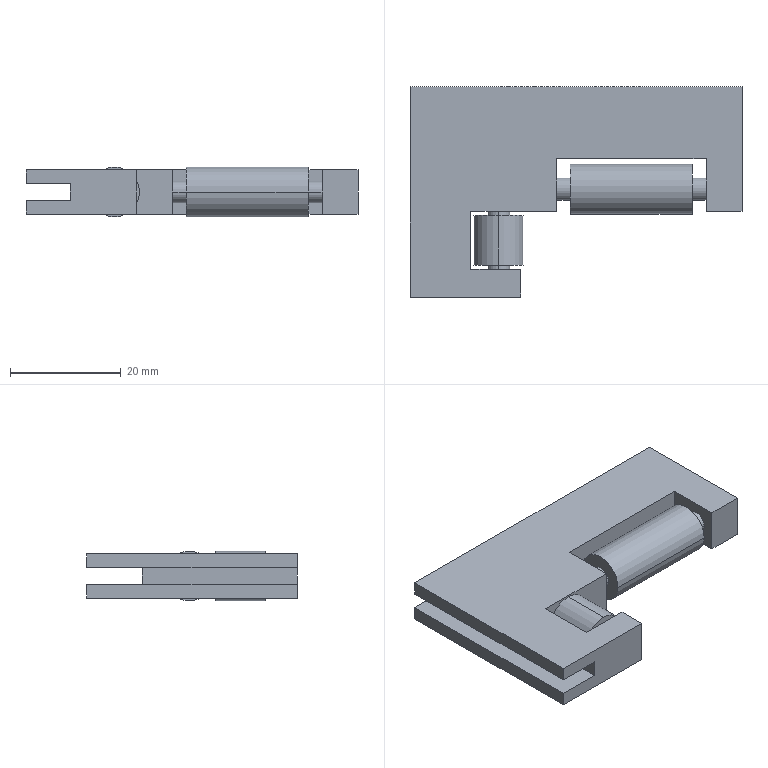Part | STEP file | T Slider Block | 3 solids | 40 faces | box 60 x 38 x 9 mm | volume 10054 mm3 | plane 28 | cylinder 12 | commonest cylinder face diameters 4 x8 9 x4
STEP:
#1=CARTESIAN_POINT('',(-41.818,-4.436,-4.5));
#2=VERTEX_POINT('',#1);
#3=CARTESIAN_POINT('',(-41.818,-4.436,4.5));
#4=VERTEX_POINT('',#3);
#5=CARTESIAN_POINT('',(-41.818,-4.436,0.));
#6=DIRECTION('',(0.,-1.,0.));
#7=DIRECTION('',(0.,0.,-1.));
#8=AXIS2_PLACEMENT_3D('',#5,#6,#7);
#9=CIRCLE('',#8,4.5);
#10=EDGE_CURVE('',#2,#4,#9,.T.);
#11=ORIENTED_EDGE('',*,*,#10,.T.);
#12=CARTESIAN_POINT('',(-41.818,-13.436,4.5));
#13=VERTEX_POINT('',#12);
#14=CARTESIAN_POINT('',(-41.818,-14.186,4.5));
#15=DIRECTION('',(0.,-1.,0.));
#16=VECTOR('',#15,1000.);
#17=LINE('',#14,#16);
#18=EDGE_CURVE('',#4,#13,#17,.T.);
#19=ORIENTED_EDGE('',*,*,#18,.T.);
#20=CARTESIAN_POINT('',(-41.818,-13.436,-4.5));
#21=VERTEX_POINT('',#20);
#22=CARTESIAN_POINT('',(-41.818,-13.436,0.));
#23=DIRECTION('',(0.,1.,0.));
#24=DIRECTION('',(0.,0.,-1.));
#25=AXIS2_PLACEMENT_3D('',#22,#23,#24);
#26=CIRCLE('',#25,4.5);
#27=EDGE_CURVE('',#13,#21,#26,.T.);
#28=ORIENTED_EDGE('',*,*,#27,.T.);
#29=CARTESIAN_POINT('',(-41.818,-14.186,-4.5));
#30=DIRECTION('',(0.,-1.,0.));
#31=VECTOR('',#30,1000.);
#32=LINE('',#29,#31);
#33=EDGE_CURVE('',#2,#21,#32,.T.);
#34=ORIENTED_EDGE('',*,*,#33,.F.);
#35=EDGE_LOOP('',(#11,#19,#28,#34));
#36=FACE_OUTER_BOUND('',#35,.T.);
#37=CARTESIAN_POINT('',(-41.818,-14.186,0.));
#38=DIRECTION('',(0.,-1.,0.));
#39=DIRECTION('',(0.,0.,-1.));
#40=AXIS2_PLACEMENT_3D('',#37,#38,#39);
#41=CYLINDRICAL_SURFACE('',#40,4.5);
#42=ADVANCED_FACE('',(#36),#41,.T.);
#43=CARTESIAN_POINT('',(-41.818,-13.436,-2.));
#44=VERTEX_POINT('',#43);
#45=CARTESIAN_POINT('',(-41.818,-13.436,2.));
#46=VERTEX_POINT('',#45);
#47=CARTESIAN_POINT('',(-41.818,-13.436,0.));
#48=DIRECTION('',(0.,-1.,0.));
#49=DIRECTION('',(0.,0.,-1.));
#50=AXIS2_PLACEMENT_3D('',#47,#48,#49);
#51=CIRCLE('',#50,2.);
#52=EDGE_CURVE('',#44,#46,#51,.T.);
#53=ORIENTED_EDGE('',*,*,#52,.T.);
#54=CARTESIAN_POINT('',(-41.818,-14.186,2.));
#55=VERTEX_POINT('',#54);
#56=CARTESIAN_POINT('',(-41.818,-14.186,2.));
#57=DIRECTION('',(0.,-1.,0.));
#58=VECTOR('',#57,1000.);
#59=LINE('',#56,#58);
#60=EDGE_CURVE('',#46,#55,#59,.T.);
#61=ORIENTED_EDGE('',*,*,#60,.T.);
#62=CARTESIAN_POINT('',(-41.818,-14.186,-2.));
#63=VERTEX_POINT('',#62);
#64=CARTESIAN_POINT('',(-41.818,-14.186,0.));
#65=DIRECTION('',(0.,1.,0.));
#66=DIRECTION('',(0.,0.,-1.));
#67=AXIS2_PLACEMENT_3D('',#64,#65,#66);
#68=CIRCLE('',#67,2.);
#69=EDGE_CURVE('',#55,#63,#68,.T.);
#70=ORIENTED_EDGE('',*,*,#69,.T.);
#71=CARTESIAN_POINT('',(-41.818,-14.186,-2.));
#72=DIRECTION('',(0.,-1.,0.));
#73=VECTOR('',#72,1000.);
#74=LINE('',#71,#73);
#75=EDGE_CURVE('',#44,#63,#74,.T.);
#76=ORIENTED_EDGE('',*,*,#75,.F.);
#77=EDGE_LOOP('',(#53,#61,#70,#76));
#78=FACE_OUTER_BOUND('',#77,.T.);
#79=CARTESIAN_POINT('',(-41.818,-14.186,0.));
#80=DIRECTION('',(0.,-1.,0.));
#81=DIRECTION('',(0.,0.,-1.));
#82=AXIS2_PLACEMENT_3D('',#79,#80,#81);
#83=CYLINDRICAL_SURFACE('',#82,2.);
#84=ADVANCED_FACE('',(#78),#83,.T.);
#85=CARTESIAN_POINT('',(-41.818,-3.686,-2.));
#86=VERTEX_POINT('',#85);
#87=CARTESIAN_POINT('',(-41.818,-3.686,2.));
#88=VERTEX_POINT('',#87);
#89=CARTESIAN_POINT('',(-41.818,-3.686,0.));
#90=DIRECTION('',(0.,-1.,0.));
#91=DIRECTION('',(0.,0.,-1.));
#92=AXIS2_PLACEMENT_3D('',#89,#90,#91);
#93=CIRCLE('',#92,2.);
#94=EDGE_CURVE('',#86,#88,#93,.T.);
#95=ORIENTED_EDGE('',*,*,#94,.T.);
#96=CARTESIAN_POINT('',(-41.818,-4.436,2.));
#97=VERTEX_POINT('',#96);
#98=CARTESIAN_POINT('',(-41.818,-14.186,2.));
#99=DIRECTION('',(0.,-1.,0.));
#100=VECTOR('',#99,1000.);
#101=LINE('',#98,#100);
#102=EDGE_CURVE('',#88,#97,#101,.T.);
#103=ORIENTED_EDGE('',*,*,#102,.T.);
#104=CARTESIAN_POINT('',(-41.818,-4.436,-2.));
#105=VERTEX_POINT('',#104);
#106=CARTESIAN_POINT('',(-41.818,-4.436,0.));
#107=DIRECTION('',(0.,1.,0.));
#108=DIRECTION('',(0.,0.,-1.));
#109=AXIS2_PLACEMENT_3D('',#106,#107,#108);
#110=CIRCLE('',#109,2.);
#111=EDGE_CURVE('',#97,#105,#110,.T.);
#112=ORIENTED_EDGE('',*,*,#111,.T.);
#113=CARTESIAN_POINT('',(-41.818,-14.186,-2.));
#114=DIRECTION('',(0.,-1.,0.));
#115=VECTOR('',#114,1000.);
#116=LINE('',#113,#115);
#117=EDGE_CURVE('',#86,#105,#116,.T.);
#118=ORIENTED_EDGE('',*,*,#117,.F.);
#119=EDGE_LOOP('',(#95,#103,#112,#118));
#120=FACE_OUTER_BOUND('',#119,.T.);
#121=CARTESIAN_POINT('',(-41.818,-14.186,0.));
#122=DIRECTION('',(0.,-1.,0.));
#123=DIRECTION('',(0.,0.,-1.));
#124=AXIS2_PLACEMENT_3D('',#121,#122,#123);
#125=CYLINDRICAL_SURFACE('',#124,2.);
#126=ADVANCED_FACE('',(#120),#125,.T.);
#127=ORIENTED_EDGE('',*,*,#18,.F.);
#128=CARTESIAN_POINT('',(-41.818,-4.436,0.));
#129=DIRECTION('',(0.,-1.,0.));
#130=DIRECTION('',(0.,0.,-1.));
#131=AXIS2_PLACEMENT_3D('',#128,#129,#130);
#132=CIRCLE('',#131,4.5);
#133=EDGE_CURVE('',#4,#2,#132,.T.);
#134=ORIENTED_EDGE('',*,*,#133,.T.);
#135=ORIENTED_EDGE('',*,*,#33,.T.);
#136=CARTESIAN_POINT('',(-41.818,-13.436,0.));
#137=DIRECTION('',(0.,1.,0.));
#138=DIRECTION('',(0.,0.,-1.));
#139=AXIS2_PLACEMENT_3D('',#136,#137,#138);
#140=CIRCLE('',#139,4.5);
#141=EDGE_CURVE('',#21,#13,#140,.T.);
#142=ORIENTED_EDGE('',*,*,#141,.T.);
#143=EDGE_LOOP('',(#127,#134,#135,#142));
#144=FACE_OUTER_BOUND('',#143,.T.);
#145=CARTESIAN_POINT('',(-41.818,-14.186,0.));
#146=DIRECTION('',(0.,-1.,0.));
#147=DIRECTION('',(0.,0.,-1.));
#148=AXIS2_PLACEMENT_3D('',#145,#146,#147);
#149=CYLINDRICAL_SURFACE('',#148,4.5);
#150=ADVANCED_FACE('',(#144),#149,.T.);
#151=ORIENTED_EDGE('',*,*,#141,.F.);
#152=ORIENTED_EDGE('',*,*,#27,.F.);
#153=EDGE_LOOP('',(#151,#152));
#154=FACE_OUTER_BOUND('',#153,.T.);
#155=ORIENTED_EDGE('',*,*,#52,.F.);
#156=CARTESIAN_POINT('',(-41.818,-13.436,0.));
#157=DIRECTION('',(0.,-1.,0.));
#158=DIRECTION('',(0.,0.,-1.));
#159=AXIS2_PLACEMENT_3D('',#156,#157,#158);
#160=CIRCLE('',#159,2.);
#161=EDGE_CURVE('',#46,#44,#160,.T.);
#162=ORIENTED_EDGE('',*,*,#161,.F.);
#163=EDGE_LOOP('',(#155,#162));
#164=FACE_BOUND('',#163,.T.);
#165=CARTESIAN_POINT('',(-46.318,-13.436,0.));
#166=DIRECTION('',(0.,1.,0.));
#167=DIRECTION('',(0.,0.,1.));
#168=AXIS2_PLACEMENT_3D('',#165,#166,#167);
#169=PLANE('',#168);
#170=ADVANCED_FACE('',(#154,#164),#169,.F.);
#171=CARTESIAN_POINT('',(-41.818,-4.436,0.));
#172=DIRECTION('',(0.,1.,0.));
#173=DIRECTION('',(0.,0.,-1.));
#174=AXIS2_PLACEMENT_3D('',#171,#172,#173);
#175=CIRCLE('',#174,2.);
#176=EDGE_CURVE('',#105,#97,#175,.T.);
#177=ORIENTED_EDGE('',*,*,#176,.F.);
#178=ORIENTED_EDGE('',*,*,#111,.F.);
#179=EDGE_LOOP('',(#177,#178));
#180=FACE_BOUND('',#179,.T.);
#181=ORIENTED_EDGE('',*,*,#10,.F.);
#182=ORIENTED_EDGE('',*,*,#133,.F.);
#183=EDGE_LOOP('',(#181,#182));
#184=FACE_OUTER_BOUND('',#183,.T.);
#185=CARTESIAN_POINT('',(-46.318,-4.436,0.));
#186=DIRECTION('',(0.,-1.,0.));
#187=DIRECTION('',(0.,0.,-1.));
#188=AXIS2_PLACEMENT_3D('',#185,#186,#187);
#189=PLANE('',#188);
#190=ADVANCED_FACE('',(#180,#184),#189,.F.);
#191=ORIENTED_EDGE('',*,*,#60,.F.);
#192=ORIENTED_EDGE('',*,*,#161,.T.);
#193=ORIENTED_EDGE('',*,*,#75,.T.);
#194=CARTESIAN_POINT('',(-41.818,-14.186,0.));
#195=DIRECTION('',(0.,1.,0.));
#196=DIRECTION('',(0.,0.,-1.));
#197=AXIS2_PLACEMENT_3D('',#194,#195,#196);
#198=CIRCLE('',#197,2.);
#199=EDGE_CURVE('',#63,#55,#198,.T.);
#200=ORIENTED_EDGE('',*,*,#199,.T.);
#201=EDGE_LOOP('',(#191,#192,#193,#200));
#202=FACE_OUTER_BOUND('',#201,.T.);
#203=CARTESIAN_POINT('',(-41.818,-14.186,0.));
#204=DIRECTION('',(0.,-1.,0.));
#205=DIRECTION('',(0.,0.,-1.));
#206=AXIS2_PLACEMENT_3D('',#203,#204,#205);
#207=CYLINDRICAL_SURFACE('',#206,2.);
#208=ADVANCED_FACE('',(#202),#207,.T.);
#209=ORIENTED_EDGE('',*,*,#102,.F.);
#210=CARTESIAN_POINT('',(-41.818,-3.686,0.));
#211=DIRECTION('',(0.,-1.,0.));
#212=DIRECTION('',(0.,0.,-1.));
#213=AXIS2_PLACEMENT_3D('',#210,#211,#212);
#214=CIRCLE('',#213,2.);
#215=EDGE_CURVE('',#88,#86,#214,.T.);
#216=ORIENTED_EDGE('',*,*,#215,.T.);
#217=ORIENTED_EDGE('',*,*,#117,.T.);
#218=ORIENTED_EDGE('',*,*,#176,.T.);
#219=EDGE_LOOP('',(#209,#216,#217,#218));
#220=FACE_OUTER_BOUND('',#219,.T.);
#221=CARTESIAN_POINT('',(-41.818,-14.186,0.));
#222=DIRECTION('',(0.,-1.,0.));
#223=DIRECTION('',(0.,0.,-1.));
#224=AXIS2_PLACEMENT_3D('',#221,#222,#223);
#225=CYLINDRICAL_SURFACE('',#224,2.);
#226=ADVANCED_FACE('',(#220),#225,.T.);
#227=ORIENTED_EDGE('',*,*,#199,.F.);
#228=ORIENTED_EDGE('',*,*,#69,.F.);
#229=EDGE_LOOP('',(#227,#228));
#230=FACE_OUTER_BOUND('',#229,.T.);
#231=CARTESIAN_POINT('',(-43.818,-14.186,0.));
#232=DIRECTION('',(0.,1.,0.));
#233=DIRECTION('',(0.,0.,1.));
#234=AXIS2_PLACEMENT_3D('',#231,#232,#233);
#235=PLANE('',#234);
#236=ADVANCED_FACE('',(#230),#235,.F.);
#237=ORIENTED_EDGE('',*,*,#94,.F.);
#238=ORIENTED_EDGE('',*,*,#215,.F.);
#239=EDGE_LOOP('',(#237,#238));
#240=FACE_OUTER_BOUND('',#239,.T.);
#241=CARTESIAN_POINT('',(-43.818,-3.686,0.));
#242=DIRECTION('',(0.,-1.,0.));
#243=DIRECTION('',(0.,0.,-1.));
#244=AXIS2_PLACEMENT_3D('',#241,#242,#243);
#245=PLANE('',#244);
#246=ADVANCED_FACE('',(#240),#245,.F.);
#247=CLOSED_SHELL('',(#42,#84,#126,#150,#170,#190,#208,#226,#236,#246));
#248=MANIFOLD_SOLID_BREP('',#247);
#249=CARTESIAN_POINT('',(-6.818,-4.186,0.));
#250=VERTEX_POINT('',#249);
#251=CARTESIAN_POINT('',(-6.818,4.814,0.));
#252=VERTEX_POINT('',#251);
#253=CARTESIAN_POINT('',(-6.818,0.3144,0.));
#254=DIRECTION('',(-1.,0.,0.));
#255=DIRECTION('',(0.,-1.,0.));
#256=AXIS2_PLACEMENT_3D('',#253,#254,#255);
#257=CIRCLE('',#256,4.5);
#258=EDGE_CURVE('',#250,#252,#257,.T.);
#259=ORIENTED_EDGE('',*,*,#258,.T.);
#260=CARTESIAN_POINT('',(-28.818,4.814,0.));
#261=VERTEX_POINT('',#260);
#262=CARTESIAN_POINT('',(-31.318,4.814,0.));
#263=DIRECTION('',(-1.,0.,0.));
#264=VECTOR('',#263,1000.);
#265=LINE('',#262,#264);
#266=EDGE_CURVE('',#252,#261,#265,.T.);
#267=ORIENTED_EDGE('',*,*,#266,.T.);
#268=CARTESIAN_POINT('',(-28.818,-4.186,0.));
#269=VERTEX_POINT('',#268);
#270=CARTESIAN_POINT('',(-28.818,0.3144,0.));
#271=DIRECTION('',(1.,0.,0.));
#272=DIRECTION('',(0.,-1.,0.));
#273=AXIS2_PLACEMENT_3D('',#270,#271,#272);
#274=CIRCLE('',#273,4.5);
#275=EDGE_CURVE('',#261,#269,#274,.T.);
#276=ORIENTED_EDGE('',*,*,#275,.T.);
#277=CARTESIAN_POINT('',(-31.318,-4.186,0.));
#278=DIRECTION('',(-1.,0.,0.));
#279=VECTOR('',#278,1000.);
#280=LINE('',#277,#279);
#281=EDGE_CURVE('',#250,#269,#280,.T.);
#282=ORIENTED_EDGE('',*,*,#281,.F.);
#283=EDGE_LOOP('',(#259,#267,#276,#282));
#284=FACE_OUTER_BOUND('',#283,.T.);
#285=CARTESIAN_POINT('',(-31.318,0.3144,0.));
#286=DIRECTION('',(-1.,0.,0.));
#287=DIRECTION('',(0.,-1.,0.));
#288=AXIS2_PLACEMENT_3D('',#285,#286,#287);
#289=CYLINDRICAL_SURFACE('',#288,4.5);
#290=ADVANCED_FACE('',(#284),#289,.T.);
#291=CARTESIAN_POINT('',(-28.818,-1.686,0.));
#292=VERTEX_POINT('',#291);
#293=CARTESIAN_POINT('',(-28.818,2.314,0.));
#294=VERTEX_POINT('',#293);
#295=CARTESIAN_POINT('',(-28.818,0.3144,0.));
#296=DIRECTION('',(-1.,0.,0.));
#297=DIRECTION('',(0.,-1.,0.));
#298=AXIS2_PLACEMENT_3D('',#295,#296,#297);
#299=CIRCLE('',#298,2.);
#300=EDGE_CURVE('',#292,#294,#299,.T.);
#301=ORIENTED_EDGE('',*,*,#300,.T.);
#302=CARTESIAN_POINT('',(-31.318,2.314,0.));
#303=VERTEX_POINT('',#302);
#304=CARTESIAN_POINT('',(-31.318,2.314,0.));
#305=DIRECTION('',(-1.,0.,0.));
#306=VECTOR('',#305,1000.);
#307=LINE('',#304,#306);
#308=EDGE_CURVE('',#294,#303,#307,.T.);
#309=ORIENTED_EDGE('',*,*,#308,.T.);
#310=CARTESIAN_POINT('',(-31.318,-1.686,0.));
#311=VERTEX_POINT('',#310);
#312=CARTESIAN_POINT('',(-31.318,0.3144,0.));
#313=DIRECTION('',(1.,0.,0.));
#314=DIRECTION('',(0.,-1.,0.));
#315=AXIS2_PLACEMENT_3D('',#312,#313,#314);
#316=CIRCLE('',#315,2.);
#317=EDGE_CURVE('',#303,#311,#316,.T.);
#318=ORIENTED_EDGE('',*,*,#317,.T.);
#319=CARTESIAN_POINT('',(-31.318,-1.686,0.));
#320=DIRECTION('',(-1.,0.,0.));
#321=VECTOR('',#320,1000.);
#322=LINE('',#319,#321);
#323=EDGE_CURVE('',#292,#311,#322,.T.);
#324=ORIENTED_EDGE('',*,*,#323,.F.);
#325=EDGE_LOOP('',(#301,#309,#318,#324));
#326=FACE_OUTER_BOUND('',#325,.T.);
#327=CARTESIAN_POINT('',(-31.318,0.3144,0.));
#328=DIRECTION('',(-1.,0.,0.));
#329=DIRECTION('',(0.,-1.,0.));
#330=AXIS2_PLACEMENT_3D('',#327,#328,#329);
#331=CYLINDRICAL_SURFACE('',#330,2.);
#332=ADVANCED_FACE('',(#326),#331,.T.);
#333=CARTESIAN_POINT('',(-4.318,-1.686,0.));
#334=VERTEX_POINT('',#333);
#335=CARTESIAN_POINT('',(-4.318,2.314,0.));
#336=VERTEX_POINT('',#335);
#337=CARTESIAN_POINT('',(-4.318,0.3144,0.));
#338=DIRECTION('',(-1.,0.,0.));
#339=DIRECTION('',(0.,-1.,0.));
#340=AXIS2_PLACEMENT_3D('',#337,#338,#339);
#341=CIRCLE('',#340,2.);
#342=EDGE_CURVE('',#334,#336,#341,.T.);
#343=ORIENTED_EDGE('',*,*,#342,.T.);
#344=CARTESIAN_POINT('',(-6.818,2.314,0.));
#345=VERTEX_POINT('',#344);
#346=CARTESIAN_POINT('',(-31.318,2.314,0.));
#347=DIRECTION('',(-1.,0.,0.));
#348=VECTOR('',#347,1000.);
#349=LINE('',#346,#348);
#350=EDGE_CURVE('',#336,#345,#349,.T.);
#351=ORIENTED_EDGE('',*,*,#350,.T.);
#352=CARTESIAN_POINT('',(-6.818,-1.686,0.));
#353=VERTEX_POINT('',#352);
#354=CARTESIAN_POINT('',(-6.818,0.3144,0.));
#355=DIRECTION('',(1.,0.,0.));
#356=DIRECTION('',(0.,-1.,0.));
#357=AXIS2_PLACEMENT_3D('',#354,#355,#356);
#358=CIRCLE('',#357,2.);
#359=EDGE_CURVE('',#345,#353,#358,.T.);
#360=ORIENTED_EDGE('',*,*,#359,.T.);
#361=CARTESIAN_POINT('',(-31.318,-1.686,0.));
#362=DIRECTION('',(-1.,0.,0.));
#363=VECTOR('',#362,1000.);
#364=LINE('',#361,#363);
#365=EDGE_CURVE('',#334,#353,#364,.T.);
#366=ORIENTED_EDGE('',*,*,#365,.F.);
#367=EDGE_LOOP('',(#343,#351,#360,#366));
#368=FACE_OUTER_BOUND('',#367,.T.);
#369=CARTESIAN_POINT('',(-31.318,0.3144,0.));
#370=DIRECTION('',(-1.,0.,0.));
#371=DIRECTION('',(0.,-1.,0.));
#372=AXIS2_PLACEMENT_3D('',#369,#370,#371);
#373=CYLINDRICAL_SURFACE('',#372,2.);
#374=ADVANCED_FACE('',(#368),#373,.T.);
#375=ORIENTED_EDGE('',*,*,#266,.F.);
#376=CARTESIAN_POINT('',(-6.818,0.3144,0.));
#377=DIRECTION('',(-1.,0.,0.));
#378=DIRECTION('',(0.,-1.,0.));
#379=AXIS2_PLACEMENT_3D('',#376,#377,#378);
#380=CIRCLE('',#379,4.5);
#381=EDGE_CURVE('',#252,#250,#380,.T.);
#382=ORIENTED_EDGE('',*,*,#381,.T.);
#383=ORIENTED_EDGE('',*,*,#281,.T.);
#384=CARTESIAN_POINT('',(-28.818,0.3144,0.));
#385=DIRECTION('',(1.,0.,0.));
#386=DIRECTION('',(0.,-1.,0.));
#387=AXIS2_PLACEMENT_3D('',#384,#385,#386);
#388=CIRCLE('',#387,4.5);
#389=EDGE_CURVE('',#269,#261,#388,.T.);
#390=ORIENTED_EDGE('',*,*,#389,.T.);
#391=EDGE_LOOP('',(#375,#382,#383,#390));
#392=FACE_OUTER_BOUND('',#391,.T.);
#393=CARTESIAN_POINT('',(-31.318,0.3144,0.));
#394=DIRECTION('',(-1.,0.,0.));
#395=DIRECTION('',(0.,-1.,0.));
#396=AXIS2_PLACEMENT_3D('',#393,#394,#395);
#397=CYLINDRICAL_SURFACE('',#396,4.5);
#398=ADVANCED_FACE('',(#392),#397,.T.);
#399=ORIENTED_EDGE('',*,*,#389,.F.);
#400=ORIENTED_EDGE('',*,*,#275,.F.);
#401=EDGE_LOOP('',(#399,#400));
#402=FACE_OUTER_BOUND('',#401,.T.);
#403=ORIENTED_EDGE('',*,*,#300,.F.);
#404=CARTESIAN_POINT('',(-28.818,0.3144,0.));
#405=DIRECTION('',(-1.,0.,0.));
#406=DIRECTION('',(0.,-1.,0.));
#407=AXIS2_PLACEMENT_3D('',#404,#405,#406);
#408=CIRCLE('',#407,2.);
#409=EDGE_CURVE('',#294,#292,#408,.T.);
#410=ORIENTED_EDGE('',*,*,#409,.F.);
#411=EDGE_LOOP('',(#403,#410));
#412=FACE_BOUND('',#411,.T.);
#413=CARTESIAN_POINT('',(-28.818,4.814,0.));
#414=DIRECTION('',(1.,0.,0.));
#415=DIRECTION('',(0.,1.,0.));
#416=AXIS2_PLACEMENT_3D('',#413,#414,#415);
#417=PLANE('',#416);
#418=ADVANCED_FACE('',(#402,#412),#417,.F.);
#419=CARTESIAN_POINT('',(-6.818,0.3144,0.));
#420=DIRECTION('',(1.,0.,0.));
#421=DIRECTION('',(0.,-1.,0.));
#422=AXIS2_PLACEMENT_3D('',#419,#420,#421);
#423=CIRCLE('',#422,2.);
#424=EDGE_CURVE('',#353,#345,#423,.T.);
#425=ORIENTED_EDGE('',*,*,#424,.F.);
#426=ORIENTED_EDGE('',*,*,#359,.F.);
#427=EDGE_LOOP('',(#425,#426));
#428=FACE_BOUND('',#427,.T.);
#429=ORIENTED_EDGE('',*,*,#258,.F.);
#430=ORIENTED_EDGE('',*,*,#381,.F.);
#431=EDGE_LOOP('',(#429,#430));
#432=FACE_OUTER_BOUND('',#431,.T.);
#433=CARTESIAN_POINT('',(-6.818,4.814,0.));
#434=DIRECTION('',(-1.,0.,0.));
#435=DIRECTION('',(0.,-1.,0.));
#436=AXIS2_PLACEMENT_3D('',#433,#434,#435);
#437=PLANE('',#436);
#438=ADVANCED_FACE('',(#428,#432),#437,.F.);
#439=ORIENTED_EDGE('',*,*,#308,.F.);
#440=ORIENTED_EDGE('',*,*,#409,.T.);
#441=ORIENTED_EDGE('',*,*,#323,.T.);
#442=CARTESIAN_POINT('',(-31.318,0.3144,0.));
#443=DIRECTION('',(1.,0.,0.));
#444=DIRECTION('',(0.,-1.,0.));
#445=AXIS2_PLACEMENT_3D('',#442,#443,#444);
#446=CIRCLE('',#445,2.);
#447=EDGE_CURVE('',#311,#303,#446,.T.);
#448=ORIENTED_EDGE('',*,*,#447,.T.);
#449=EDGE_LOOP('',(#439,#440,#441,#448));
#450=FACE_OUTER_BOUND('',#449,.T.);
#451=CARTESIAN_POINT('',(-31.318,0.3144,0.));
#452=DIRECTION('',(-1.,0.,0.));
#453=DIRECTION('',(0.,-1.,0.));
#454=AXIS2_PLACEMENT_3D('',#451,#452,#453);
#455=CYLINDRICAL_SURFACE('',#454,2.);
#456=ADVANCED_FACE('',(#450),#455,.T.);
#457=ORIENTED_EDGE('',*,*,#350,.F.);
#458=CARTESIAN_POINT('',(-4.318,0.3144,0.));
#459=DIRECTION('',(-1.,0.,0.));
#460=DIRECTION('',(0.,-1.,0.));
#461=AXIS2_PLACEMENT_3D('',#458,#459,#460);
#462=CIRCLE('',#461,2.);
#463=EDGE_CURVE('',#336,#334,#462,.T.);
#464=ORIENTED_EDGE('',*,*,#463,.T.);
#465=ORIENTED_EDGE('',*,*,#365,.T.);
#466=ORIENTED_EDGE('',*,*,#424,.T.);
#467=EDGE_LOOP('',(#457,#464,#465,#466));
#468=FACE_OUTER_BOUND('',#467,.T.);
#469=CARTESIAN_POINT('',(-31.318,0.3144,0.));
#470=DIRECTION('',(-1.,0.,0.));
#471=DIRECTION('',(0.,-1.,0.));
#472=AXIS2_PLACEMENT_3D('',#469,#470,#471);
#473=CYLINDRICAL_SURFACE('',#472,2.);
#474=ADVANCED_FACE('',(#468),#473,.T.);
#475=ORIENTED_EDGE('',*,*,#447,.F.);
#476=ORIENTED_EDGE('',*,*,#317,.F.);
#477=EDGE_LOOP('',(#475,#476));
#478=FACE_OUTER_BOUND('',#477,.T.);
#479=CARTESIAN_POINT('',(-31.318,2.314,0.));
#480=DIRECTION('',(1.,0.,0.));
#481=DIRECTION('',(0.,1.,0.));
#482=AXIS2_PLACEMENT_3D('',#479,#480,#481);
#483=PLANE('',#482);
#484=ADVANCED_FACE('',(#478),#483,.F.);
#485=ORIENTED_EDGE('',*,*,#342,.F.);
#486=ORIENTED_EDGE('',*,*,#463,.F.);
#487=EDGE_LOOP('',(#485,#486));
#488=FACE_OUTER_BOUND('',#487,.T.);
#489=CARTESIAN_POINT('',(-4.318,2.314,0.));
#490=DIRECTION('',(-1.,0.,0.));
#491=DIRECTION('',(0.,-1.,0.));
#492=AXIS2_PLACEMENT_3D('',#489,#490,#491);
#493=PLANE('',#492);
#494=ADVANCED_FACE('',(#488),#493,.F.);
#495=CLOSED_SHELL('',(#290,#332,#374,#398,#418,#438,#456,#474,#484,#494));
#496=MANIFOLD_SOLID_BREP('',#495);
#497=CARTESIAN_POINT('',(-37.818,-19.186,4.));
#498=VERTEX_POINT('',#497);
#499=CARTESIAN_POINT('',(-57.818,-19.186,4.));
#500=VERTEX_POINT('',#499);
#501=CARTESIAN_POINT('',(0.,-19.186,4.));
#502=DIRECTION('',(-1.,0.,0.));
#503=VECTOR('',#502,1000.);
#504=LINE('',#501,#503);
#505=EDGE_CURVE('',#498,#500,#504,.T.);
#506=ORIENTED_EDGE('',*,*,#505,.F.);
#507=CARTESIAN_POINT('',(-37.818,-14.186,4.));
#508=VERTEX_POINT('',#507);
#509=CARTESIAN_POINT('',(-37.818,0.,4.));
#510=DIRECTION('',(0.,-1.,0.));
#511=VECTOR('',#510,1000.);
#512=LINE('',#509,#511);
#513=EDGE_CURVE('',#508,#498,#512,.T.);
#514=ORIENTED_EDGE('',*,*,#513,.F.);
#515=CARTESIAN_POINT('',(-46.818,-14.186,4.));
#516=VERTEX_POINT('',#515);
#517=CARTESIAN_POINT('',(0.,-14.186,4.));
#518=DIRECTION('',(1.,0.,0.));
#519=VECTOR('',#518,1000.);
#520=LINE('',#517,#519);
#521=EDGE_CURVE('',#516,#508,#520,.T.);
#522=ORIENTED_EDGE('',*,*,#521,.F.);
#523=CARTESIAN_POINT('',(-46.818,-3.686,4.));
#524=VERTEX_POINT('',#523);
#525=CARTESIAN_POINT('',(-46.818,0.,4.));
#526=DIRECTION('',(0.,-1.,0.));
#527=VECTOR('',#526,1000.);
#528=LINE('',#525,#527);
#529=EDGE_CURVE('',#524,#516,#528,.T.);
#530=ORIENTED_EDGE('',*,*,#529,.F.);
#531=CARTESIAN_POINT('',(-31.318,-3.686,4.));
#532=VERTEX_POINT('',#531);
#533=CARTESIAN_POINT('',(0.,-3.686,4.));
#534=DIRECTION('',(-1.,0.,0.));
#535=VECTOR('',#534,1000.);
#536=LINE('',#533,#535);
#537=EDGE_CURVE('',#532,#524,#536,.T.);
#538=ORIENTED_EDGE('',*,*,#537,.F.);
#539=CARTESIAN_POINT('',(-31.318,5.814,4.));
#540=VERTEX_POINT('',#539);
#541=CARTESIAN_POINT('',(-31.318,0.,4.));
#542=DIRECTION('',(0.,-1.,0.));
#543=VECTOR('',#542,1000.);
#544=LINE('',#541,#543);
#545=EDGE_CURVE('',#540,#532,#544,.T.);
#546=ORIENTED_EDGE('',*,*,#545,.F.);
#547=CARTESIAN_POINT('',(-4.318,5.814,4.));
#548=VERTEX_POINT('',#547);
#549=CARTESIAN_POINT('',(0.,5.814,4.));
#550=DIRECTION('',(-1.,0.,0.));
#551=VECTOR('',#550,1000.);
#552=LINE('',#549,#551);
#553=EDGE_CURVE('',#548,#540,#552,.T.);
#554=ORIENTED_EDGE('',*,*,#553,.F.);
#555=CARTESIAN_POINT('',(-4.318,-3.686,4.));
#556=VERTEX_POINT('',#555);
#557=CARTESIAN_POINT('',(-4.318,0.,4.));
#558=DIRECTION('',(0.,1.,0.));
#559=VECTOR('',#558,1000.);
#560=LINE('',#557,#559);
#561=EDGE_CURVE('',#556,#548,#560,.T.);
#562=ORIENTED_EDGE('',*,*,#561,.F.);
#563=CARTESIAN_POINT('',(2.182,-3.686,4.));
#564=VERTEX_POINT('',#563);
#565=CARTESIAN_POINT('',(0.,-3.686,4.));
#566=DIRECTION('',(-1.,0.,0.));
#567=VECTOR('',#566,1000.);
#568=LINE('',#565,#567);
#569=EDGE_CURVE('',#564,#556,#568,.T.);
#570=ORIENTED_EDGE('',*,*,#569,.F.);
#571=CARTESIAN_POINT('',(2.182,18.814,4.));
#572=VERTEX_POINT('',#571);
#573=CARTESIAN_POINT('',(2.182,0.,4.));
#574=DIRECTION('',(0.,-1.,0.));
#575=VECTOR('',#574,1000.);
#576=LINE('',#573,#575);
#577=EDGE_CURVE('',#572,#564,#576,.T.);
#578=ORIENTED_EDGE('',*,*,#577,.F.);
#579=CARTESIAN_POINT('',(-57.818,18.814,4.));
#580=VERTEX_POINT('',#579);
#581=CARTESIAN_POINT('',(0.,18.814,4.));
#582=DIRECTION('',(1.,0.,0.));
#583=VECTOR('',#582,1000.);
#584=LINE('',#581,#583);
#585=EDGE_CURVE('',#580,#572,#584,.T.);
#586=ORIENTED_EDGE('',*,*,#585,.F.);
#587=CARTESIAN_POINT('',(-57.818,0.,4.));
#588=DIRECTION('',(0.,1.,0.));
#589=VECTOR('',#588,1000.);
#590=LINE('',#587,#589);
#591=EDGE_CURVE('',#500,#580,#590,.T.);
#592=ORIENTED_EDGE('',*,*,#591,.F.);
#593=EDGE_LOOP('',(#506,#514,#522,#530,#538,#546,#554,#562,#570,#578,#586,#592));
#594=FACE_OUTER_BOUND('',#593,.T.);
#595=CARTESIAN_POINT('',(0.,0.,4.));
#596=DIRECTION('',(0.,0.,-1.));
#597=DIRECTION('',(-1.,0.,0.));
#598=AXIS2_PLACEMENT_3D('',#595,#596,#597);
#599=PLANE('',#598);
#600=ADVANCED_FACE('',(#594),#599,.F.);
#601=CARTESIAN_POINT('',(-57.818,-19.186,1.5));
#602=VERTEX_POINT('',#601);
#603=CARTESIAN_POINT('',(-57.818,-19.186,4.));
#604=DIRECTION('',(0.,0.,-1.));
#605=VECTOR('',#604,1000.);
#606=LINE('',#603,#605);
#607=EDGE_CURVE('',#500,#602,#606,.T.);
#608=ORIENTED_EDGE('',*,*,#607,.F.);
#609=ORIENTED_EDGE('',*,*,#591,.T.);
#610=CARTESIAN_POINT('',(-57.818,18.814,1.5));
#611=VERTEX_POINT('',#610);
#612=CARTESIAN_POINT('',(-57.818,18.814,4.));
#613=DIRECTION('',(0.,0.,1.));
#614=VECTOR('',#613,1000.);
#615=LINE('',#612,#614);
#616=EDGE_CURVE('',#611,#580,#615,.T.);
#617=ORIENTED_EDGE('',*,*,#616,.F.);
#618=CARTESIAN_POINT('',(-57.818,-19.186,1.5));
#619=DIRECTION('',(0.,1.,0.));
#620=VECTOR('',#619,1000.);
#621=LINE('',#618,#620);
#622=EDGE_CURVE('',#602,#611,#621,.T.);
#623=ORIENTED_EDGE('',*,*,#622,.F.);
#624=EDGE_LOOP('',(#608,#609,#617,#623));
#625=FACE_OUTER_BOUND('',#624,.T.);
#626=CARTESIAN_POINT('',(-57.818,-19.186,4.));
#627=DIRECTION('',(1.,0.,0.));
#628=DIRECTION('',(0.,0.,-1.));
#629=AXIS2_PLACEMENT_3D('',#626,#627,#628);
#630=PLANE('',#629);
#631=ADVANCED_FACE('',(#625),#630,.F.);
#632=CARTESIAN_POINT('',(-57.818,-19.186,-1.5));
#633=VERTEX_POINT('',#632);
#634=CARTESIAN_POINT('',(-49.818,-19.186,-1.5));
#635=VERTEX_POINT('',#634);
#636=CARTESIAN_POINT('',(-37.818,-19.186,-1.5));
#637=DIRECTION('',(1.,0.,0.));
#638=VECTOR('',#637,1000.);
#639=LINE('',#636,#638);
#640=EDGE_CURVE('',#633,#635,#639,.T.);
#641=ORIENTED_EDGE('',*,*,#640,.F.);
#642=CARTESIAN_POINT('',(-57.818,-19.186,-4.));
#643=VERTEX_POINT('',#642);
#644=CARTESIAN_POINT('',(-57.818,-19.186,4.));
#645=DIRECTION('',(0.,0.,1.));
#646=VECTOR('',#645,1000.);
#647=LINE('',#644,#646);
#648=EDGE_CURVE('',#643,#633,#647,.T.);
#649=ORIENTED_EDGE('',*,*,#648,.F.);
#650=CARTESIAN_POINT('',(-37.818,-19.186,-4.));
#651=VERTEX_POINT('',#650);
#652=CARTESIAN_POINT('',(-37.818,-19.186,-4.));
#653=DIRECTION('',(-1.,0.,0.));
#654=VECTOR('',#653,1000.);
#655=LINE('',#652,#654);
#656=EDGE_CURVE('',#651,#643,#655,.T.);
#657=ORIENTED_EDGE('',*,*,#656,.F.);
#658=CARTESIAN_POINT('',(-37.818,-19.186,4.));
#659=DIRECTION('',(0.,0.,-1.));
#660=VECTOR('',#659,1000.);
#661=LINE('',#658,#660);
#662=EDGE_CURVE('',#498,#651,#661,.T.);
#663=ORIENTED_EDGE('',*,*,#662,.F.);
#664=ORIENTED_EDGE('',*,*,#505,.T.);
#665=ORIENTED_EDGE('',*,*,#607,.T.);
#666=CARTESIAN_POINT('',(-49.818,-19.186,1.5));
#667=VERTEX_POINT('',#666);
#668=CARTESIAN_POINT('',(-37.818,-19.186,1.5));
#669=DIRECTION('',(-1.,0.,0.));
#670=VECTOR('',#669,1000.);
#671=LINE('',#668,#670);
#672=EDGE_CURVE('',#667,#602,#671,.T.);
#673=ORIENTED_EDGE('',*,*,#672,.F.);
#674=CARTESIAN_POINT('',(-49.818,-19.186,4.));
#675=DIRECTION('',(0.,0.,1.));
#676=VECTOR('',#675,1000.);
#677=LINE('',#674,#676);
#678=EDGE_CURVE('',#635,#667,#677,.T.);
#679=ORIENTED_EDGE('',*,*,#678,.F.);
#680=EDGE_LOOP('',(#641,#649,#657,#663,#664,#665,#673,#679));
#681=FACE_OUTER_BOUND('',#680,.T.);
#682=CARTESIAN_POINT('',(-37.818,-19.186,4.));
#683=DIRECTION('',(0.,1.,0.));
#684=DIRECTION('',(-1.,0.,0.));
#685=AXIS2_PLACEMENT_3D('',#682,#683,#684);
#686=PLANE('',#685);
#687=ADVANCED_FACE('',(#681),#686,.F.);
#688=CARTESIAN_POINT('',(-37.818,-14.186,-4.));
#689=VERTEX_POINT('',#688);
#690=CARTESIAN_POINT('',(-37.818,-14.186,4.));
#691=DIRECTION('',(0.,0.,-1.));
#692=VECTOR('',#691,1000.);
#693=LINE('',#690,#692);
#694=EDGE_CURVE('',#508,#689,#693,.T.);
#695=ORIENTED_EDGE('',*,*,#694,.F.);
#696=ORIENTED_EDGE('',*,*,#513,.T.);
#697=ORIENTED_EDGE('',*,*,#662,.T.);
#698=CARTESIAN_POINT('',(-37.818,-14.186,-4.));
#699=DIRECTION('',(0.,-1.,0.));
#700=VECTOR('',#699,1000.);
#701=LINE('',#698,#700);
#702=EDGE_CURVE('',#689,#651,#701,.T.);
#703=ORIENTED_EDGE('',*,*,#702,.F.);
#704=EDGE_LOOP('',(#695,#696,#697,#703));
#705=FACE_OUTER_BOUND('',#704,.T.);
#706=CARTESIAN_POINT('',(-37.818,-14.186,4.));
#707=DIRECTION('',(-1.,0.,0.));
#708=DIRECTION('',(0.,0.,1.));
#709=AXIS2_PLACEMENT_3D('',#706,#707,#708);
#710=PLANE('',#709);
#711=ADVANCED_FACE('',(#705),#710,.F.);
#712=CARTESIAN_POINT('',(-46.818,-14.186,-4.));
#713=VERTEX_POINT('',#712);
#714=CARTESIAN_POINT('',(-46.818,-14.186,4.));
#715=DIRECTION('',(0.,0.,-1.));
#716=VECTOR('',#715,1000.);
#717=LINE('',#714,#716);
#718=EDGE_CURVE('',#516,#713,#717,.T.);
#719=ORIENTED_EDGE('',*,*,#718,.F.);
#720=ORIENTED_EDGE('',*,*,#521,.T.);
#721=ORIENTED_EDGE('',*,*,#694,.T.);
#722=CARTESIAN_POINT('',(-37.818,-14.186,-4.));
#723=DIRECTION('',(1.,0.,0.));
#724=VECTOR('',#723,1000.);
#725=LINE('',#722,#724);
#726=EDGE_CURVE('',#713,#689,#725,.T.);
#727=ORIENTED_EDGE('',*,*,#726,.F.);
#728=EDGE_LOOP('',(#719,#720,#721,#727));
#729=FACE_OUTER_BOUND('',#728,.T.);
#730=CARTESIAN_POINT('',(-37.818,-14.186,4.));
#731=DIRECTION('',(0.,-1.,0.));
#732=DIRECTION('',(0.,0.,-1.));
#733=AXIS2_PLACEMENT_3D('',#730,#731,#732);
#734=PLANE('',#733);
#735=ADVANCED_FACE('',(#729),#734,.F.);
#736=CARTESIAN_POINT('',(-46.818,-3.686,-4.));
#737=VERTEX_POINT('',#736);
#738=CARTESIAN_POINT('',(-46.818,-3.686,4.));
#739=DIRECTION('',(0.,0.,-1.));
#740=VECTOR('',#739,1000.);
#741=LINE('',#738,#740);
#742=EDGE_CURVE('',#524,#737,#741,.T.);
#743=ORIENTED_EDGE('',*,*,#742,.F.);
#744=ORIENTED_EDGE('',*,*,#529,.T.);
#745=ORIENTED_EDGE('',*,*,#718,.T.);
#746=CARTESIAN_POINT('',(-46.818,-14.186,-4.));
#747=DIRECTION('',(0.,-1.,0.));
#748=VECTOR('',#747,1000.);
#749=LINE('',#746,#748);
#750=EDGE_CURVE('',#737,#713,#749,.T.);
#751=ORIENTED_EDGE('',*,*,#750,.F.);
#752=EDGE_LOOP('',(#743,#744,#745,#751));
#753=FACE_OUTER_BOUND('',#752,.T.);
#754=CARTESIAN_POINT('',(-46.818,-14.186,4.));
#755=DIRECTION('',(-1.,0.,0.));
#756=DIRECTION('',(0.,0.,1.));
#757=AXIS2_PLACEMENT_3D('',#754,#755,#756);
#758=PLANE('',#757);
#759=ADVANCED_FACE('',(#753),#758,.F.);
#760=CARTESIAN_POINT('',(-31.318,-3.686,-4.));
#761=VERTEX_POINT('',#760);
#762=CARTESIAN_POINT('',(-31.318,-3.686,4.));
#763=DIRECTION('',(0.,0.,-1.));
#764=VECTOR('',#763,1000.);
#765=LINE('',#762,#764);
#766=EDGE_CURVE('',#532,#761,#765,.T.);
#767=ORIENTED_EDGE('',*,*,#766,.F.);
#768=ORIENTED_EDGE('',*,*,#537,.T.);
#769=ORIENTED_EDGE('',*,*,#742,.T.);
#770=CARTESIAN_POINT('',(-31.318,-3.686,-4.));
#771=DIRECTION('',(-1.,0.,0.));
#772=VECTOR('',#771,1000.);
#773=LINE('',#770,#772);
#774=EDGE_CURVE('',#761,#737,#773,.T.);
#775=ORIENTED_EDGE('',*,*,#774,.F.);
#776=EDGE_LOOP('',(#767,#768,#769,#775));
#777=FACE_OUTER_BOUND('',#776,.T.);
#778=CARTESIAN_POINT('',(-31.318,-3.686,4.));
#779=DIRECTION('',(0.,1.,0.));
#780=DIRECTION('',(-1.,0.,0.));
#781=AXIS2_PLACEMENT_3D('',#778,#779,#780);
#782=PLANE('',#781);
#783=ADVANCED_FACE('',(#777),#782,.F.);
#784=CARTESIAN_POINT('',(-31.318,5.814,-4.));
#785=VERTEX_POINT('',#784);
#786=CARTESIAN_POINT('',(-31.318,5.814,4.));
#787=DIRECTION('',(0.,0.,-1.));
#788=VECTOR('',#787,1000.);
#789=LINE('',#786,#788);
#790=EDGE_CURVE('',#540,#785,#789,.T.);
#791=ORIENTED_EDGE('',*,*,#790,.F.);
#792=ORIENTED_EDGE('',*,*,#545,.T.);
#793=ORIENTED_EDGE('',*,*,#766,.T.);
#794=CARTESIAN_POINT('',(-31.318,5.814,-4.));
#795=DIRECTION('',(0.,-1.,0.));
#796=VECTOR('',#795,1000.);
#797=LINE('',#794,#796);
#798=EDGE_CURVE('',#785,#761,#797,.T.);
#799=ORIENTED_EDGE('',*,*,#798,.F.);
#800=EDGE_LOOP('',(#791,#792,#793,#799));
#801=FACE_OUTER_BOUND('',#800,.T.);
#802=CARTESIAN_POINT('',(-31.318,5.814,4.));
#803=DIRECTION('',(-1.,0.,0.));
#804=DIRECTION('',(0.,0.,1.));
#805=AXIS2_PLACEMENT_3D('',#802,#803,#804);
#806=PLANE('',#805);
#807=ADVANCED_FACE('',(#801),#806,.F.);
#808=CARTESIAN_POINT('',(-4.318,5.814,-4.));
#809=VERTEX_POINT('',#808);
#810=CARTESIAN_POINT('',(-4.318,5.814,4.));
#811=DIRECTION('',(0.,0.,-1.));
#812=VECTOR('',#811,1000.);
#813=LINE('',#810,#812);
#814=EDGE_CURVE('',#548,#809,#813,.T.);
#815=ORIENTED_EDGE('',*,*,#814,.F.);
#816=ORIENTED_EDGE('',*,*,#553,.T.);
#817=ORIENTED_EDGE('',*,*,#790,.T.);
#818=CARTESIAN_POINT('',(-4.318,5.814,-4.));
#819=DIRECTION('',(-1.,0.,0.));
#820=VECTOR('',#819,1000.);
#821=LINE('',#818,#820);
#822=EDGE_CURVE('',#809,#785,#821,.T.);
#823=ORIENTED_EDGE('',*,*,#822,.F.);
#824=EDGE_LOOP('',(#815,#816,#817,#823));
#825=FACE_OUTER_BOUND('',#824,.T.);
#826=CARTESIAN_POINT('',(-4.318,5.814,4.));
#827=DIRECTION('',(0.,1.,0.));
#828=DIRECTION('',(-1.,0.,0.));
#829=AXIS2_PLACEMENT_3D('',#826,#827,#828);
#830=PLANE('',#829);
#831=ADVANCED_FACE('',(#825),#830,.F.);
#832=CARTESIAN_POINT('',(-4.318,-3.686,-4.));
#833=VERTEX_POINT('',#832);
#834=CARTESIAN_POINT('',(-4.318,-3.686,4.));
#835=DIRECTION('',(0.,0.,-1.));
#836=VECTOR('',#835,1000.);
#837=LINE('',#834,#836);
#838=EDGE_CURVE('',#556,#833,#837,.T.);
#839=ORIENTED_EDGE('',*,*,#838,.F.);
#840=ORIENTED_EDGE('',*,*,#561,.T.);
#841=ORIENTED_EDGE('',*,*,#814,.T.);
#842=CARTESIAN_POINT('',(-4.318,-3.686,-4.));
#843=DIRECTION('',(0.,1.,0.));
#844=VECTOR('',#843,1000.);
#845=LINE('',#842,#844);
#846=EDGE_CURVE('',#833,#809,#845,.T.);
#847=ORIENTED_EDGE('',*,*,#846,.F.);
#848=EDGE_LOOP('',(#839,#840,#841,#847));
#849=FACE_OUTER_BOUND('',#848,.T.);
#850=CARTESIAN_POINT('',(-4.318,-3.686,4.));
#851=DIRECTION('',(1.,0.,0.));
#852=DIRECTION('',(0.,0.,-1.));
#853=AXIS2_PLACEMENT_3D('',#850,#851,#852);
#854=PLANE('',#853);
#855=ADVANCED_FACE('',(#849),#854,.F.);
#856=CARTESIAN_POINT('',(2.182,-3.686,-4.));
#857=VERTEX_POINT('',#856);
#858=CARTESIAN_POINT('',(2.182,-3.686,4.));
#859=DIRECTION('',(0.,0.,-1.));
#860=VECTOR('',#859,1000.);
#861=LINE('',#858,#860);
#862=EDGE_CURVE('',#564,#857,#861,.T.);
#863=ORIENTED_EDGE('',*,*,#862,.F.);
#864=ORIENTED_EDGE('',*,*,#569,.T.);
#865=ORIENTED_EDGE('',*,*,#838,.T.);
#866=CARTESIAN_POINT('',(2.182,-3.686,-4.));
#867=DIRECTION('',(-1.,0.,0.));
#868=VECTOR('',#867,1000.);
#869=LINE('',#866,#868);
#870=EDGE_CURVE('',#857,#833,#869,.T.);
#871=ORIENTED_EDGE('',*,*,#870,.F.);
#872=EDGE_LOOP('',(#863,#864,#865,#871));
#873=FACE_OUTER_BOUND('',#872,.T.);
#874=CARTESIAN_POINT('',(2.182,-3.686,4.));
#875=DIRECTION('',(0.,1.,0.));
#876=DIRECTION('',(-1.,0.,0.));
#877=AXIS2_PLACEMENT_3D('',#874,#875,#876);
#878=PLANE('',#877);
#879=ADVANCED_FACE('',(#873),#878,.F.);
#880=CARTESIAN_POINT('',(2.182,8.814,-1.5));
#881=VERTEX_POINT('',#880);
#882=CARTESIAN_POINT('',(2.182,18.814,-1.5));
#883=VERTEX_POINT('',#882);
#884=CARTESIAN_POINT('',(2.182,18.814,-1.5));
#885=DIRECTION('',(0.,1.,0.));
#886=VECTOR('',#885,1000.);
#887=LINE('',#884,#886);
#888=EDGE_CURVE('',#881,#883,#887,.T.);
#889=ORIENTED_EDGE('',*,*,#888,.F.);
#890=CARTESIAN_POINT('',(2.182,8.814,1.5));
#891=VERTEX_POINT('',#890);
#892=CARTESIAN_POINT('',(2.182,8.814,4.));
#893=DIRECTION('',(0.,0.,-1.));
#894=VECTOR('',#893,1000.);
#895=LINE('',#892,#894);
#896=EDGE_CURVE('',#891,#881,#895,.T.);
#897=ORIENTED_EDGE('',*,*,#896,.F.);
#898=CARTESIAN_POINT('',(2.182,18.814,1.5));
#899=VERTEX_POINT('',#898);
#900=CARTESIAN_POINT('',(2.182,18.814,1.5));
#901=DIRECTION('',(0.,-1.,0.));
#902=VECTOR('',#901,1000.);
#903=LINE('',#900,#902);
#904=EDGE_CURVE('',#899,#891,#903,.T.);
#905=ORIENTED_EDGE('',*,*,#904,.F.);
#906=CARTESIAN_POINT('',(2.182,18.814,4.));
#907=DIRECTION('',(0.,0.,-1.));
#908=VECTOR('',#907,1000.);
#909=LINE('',#906,#908);
#910=EDGE_CURVE('',#572,#899,#909,.T.);
#911=ORIENTED_EDGE('',*,*,#910,.F.);
#912=ORIENTED_EDGE('',*,*,#577,.T.);
#913=ORIENTED_EDGE('',*,*,#862,.T.);
#914=CARTESIAN_POINT('',(2.182,18.814,-4.));
#915=VERTEX_POINT('',#914);
#916=CARTESIAN_POINT('',(2.182,18.814,-4.));
#917=DIRECTION('',(0.,-1.,0.));
#918=VECTOR('',#917,1000.);
#919=LINE('',#916,#918);
#920=EDGE_CURVE('',#915,#857,#919,.T.);
#921=ORIENTED_EDGE('',*,*,#920,.F.);
#922=CARTESIAN_POINT('',(2.182,18.814,4.));
#923=DIRECTION('',(0.,0.,-1.));
#924=VECTOR('',#923,1000.);
#925=LINE('',#922,#924);
#926=EDGE_CURVE('',#883,#915,#925,.T.);
#927=ORIENTED_EDGE('',*,*,#926,.F.);
#928=EDGE_LOOP('',(#889,#897,#905,#911,#912,#913,#921,#927));
#929=FACE_OUTER_BOUND('',#928,.T.);
#930=CARTESIAN_POINT('',(2.182,18.814,4.));
#931=DIRECTION('',(-1.,0.,0.));
#932=DIRECTION('',(0.,-1.,0.));
#933=AXIS2_PLACEMENT_3D('',#930,#931,#932);
#934=PLANE('',#933);
#935=ADVANCED_FACE('',(#929),#934,.F.);
#936=CARTESIAN_POINT('',(-57.818,18.814,1.5));
#937=DIRECTION('',(1.,0.,0.));
#938=VECTOR('',#937,1000.);
#939=LINE('',#936,#938);
#940=EDGE_CURVE('',#611,#899,#939,.T.);
#941=ORIENTED_EDGE('',*,*,#940,.F.);
#942=ORIENTED_EDGE('',*,*,#616,.T.);
#943=ORIENTED_EDGE('',*,*,#585,.T.);
#944=ORIENTED_EDGE('',*,*,#910,.T.);
#945=EDGE_LOOP('',(#941,#942,#943,#944));
#946=FACE_OUTER_BOUND('',#945,.T.);
#947=CARTESIAN_POINT('',(-57.818,18.814,4.));
#948=DIRECTION('',(0.,-1.,0.));
#949=DIRECTION('',(0.,0.,-1.));
#950=AXIS2_PLACEMENT_3D('',#947,#948,#949);
#951=PLANE('',#950);
#952=ADVANCED_FACE('',(#946),#951,.F.);
#953=ORIENTED_EDGE('',*,*,#904,.T.);
#954=CARTESIAN_POINT('',(-49.818,8.814,1.5));
#955=VERTEX_POINT('',#954);
#956=CARTESIAN_POINT('',(-57.818,8.814,1.5));
#957=DIRECTION('',(1.,0.,0.));
#958=VECTOR('',#957,1000.);
#959=LINE('',#956,#958);
#960=EDGE_CURVE('',#955,#891,#959,.T.);
#961=ORIENTED_EDGE('',*,*,#960,.F.);
#962=CARTESIAN_POINT('',(-49.818,8.814,1.5));
#963=DIRECTION('',(0.,1.,0.));
#964=VECTOR('',#963,1000.);
#965=LINE('',#962,#964);
#966=EDGE_CURVE('',#667,#955,#965,.T.);
#967=ORIENTED_EDGE('',*,*,#966,.F.);
#968=ORIENTED_EDGE('',*,*,#672,.T.);
#969=ORIENTED_EDGE('',*,*,#622,.T.);
#970=ORIENTED_EDGE('',*,*,#940,.T.);
#971=EDGE_LOOP('',(#953,#961,#967,#968,#969,#970));
#972=FACE_OUTER_BOUND('',#971,.T.);
#973=CARTESIAN_POINT('',(-57.818,8.814,1.5));
#974=DIRECTION('',(0.,0.,1.));
#975=DIRECTION('',(1.,0.,0.));
#976=AXIS2_PLACEMENT_3D('',#973,#974,#975);
#977=PLANE('',#976);
#978=ADVANCED_FACE('',(#972),#977,.F.);
#979=ORIENTED_EDGE('',*,*,#966,.T.);
#980=CARTESIAN_POINT('',(-49.818,8.814,-1.5));
#981=VERTEX_POINT('',#980);
#982=CARTESIAN_POINT('',(-49.818,8.814,0.));
#983=DIRECTION('',(0.,0.,-1.));
#984=VECTOR('',#983,1000.);
#985=LINE('',#982,#984);
#986=EDGE_CURVE('',#955,#981,#985,.T.);
#987=ORIENTED_EDGE('',*,*,#986,.T.);
#988=CARTESIAN_POINT('',(-49.818,0.,-1.5));
#989=DIRECTION('',(0.,-1.,0.));
#990=VECTOR('',#989,1000.);
#991=LINE('',#988,#990);
#992=EDGE_CURVE('',#981,#635,#991,.T.);
#993=ORIENTED_EDGE('',*,*,#992,.T.);
#994=ORIENTED_EDGE('',*,*,#678,.T.);
#995=EDGE_LOOP('',(#979,#987,#993,#994));
#996=FACE_OUTER_BOUND('',#995,.T.);
#997=CARTESIAN_POINT('',(-49.818,0.,0.));
#998=DIRECTION('',(-1.,0.,0.));
#999=DIRECTION('',(0.,0.,1.));
#1000=AXIS2_PLACEMENT_3D('',#997,#998,#999);
#1001=PLANE('',#1000);
#1002=ADVANCED_FACE('',(#996),#1001,.T.);
#1003=ORIENTED_EDGE('',*,*,#640,.T.);
#1004=ORIENTED_EDGE('',*,*,#992,.F.);
#1005=CARTESIAN_POINT('',(-57.818,8.814,-1.5));
#1006=DIRECTION('',(-1.,0.,0.));
#1007=VECTOR('',#1006,1000.);
#1008=LINE('',#1005,#1007);
#1009=EDGE_CURVE('',#881,#981,#1008,.T.);
#1010=ORIENTED_EDGE('',*,*,#1009,.F.);
#1011=ORIENTED_EDGE('',*,*,#888,.T.);
#1012=CARTESIAN_POINT('',(-57.818,18.814,-1.5));
#1013=VERTEX_POINT('',#1012);
#1014=CARTESIAN_POINT('',(-57.818,18.814,-1.5));
#1015=DIRECTION('',(1.,0.,0.));
#1016=VECTOR('',#1015,1000.);
#1017=LINE('',#1014,#1016);
#1018=EDGE_CURVE('',#1013,#883,#1017,.T.);
#1019=ORIENTED_EDGE('',*,*,#1018,.F.);
#1020=CARTESIAN_POINT('',(-57.818,8.814,-1.5));
#1021=DIRECTION('',(0.,1.,0.));
#1022=VECTOR('',#1021,1000.);
#1023=LINE('',#1020,#1022);
#1024=EDGE_CURVE('',#633,#1013,#1023,.T.);
#1025=ORIENTED_EDGE('',*,*,#1024,.F.);
#1026=EDGE_LOOP('',(#1003,#1004,#1010,#1011,#1019,#1025));
#1027=FACE_OUTER_BOUND('',#1026,.T.);
#1028=CARTESIAN_POINT('',(-57.818,8.814,-1.5));
#1029=DIRECTION('',(0.,0.,-1.));
#1030=DIRECTION('',(-1.,0.,0.));
#1031=AXIS2_PLACEMENT_3D('',#1028,#1029,#1030);
#1032=PLANE('',#1031);
#1033=ADVANCED_FACE('',(#1027),#1032,.F.);
#1034=ORIENTED_EDGE('',*,*,#1024,.T.);
#1035=CARTESIAN_POINT('',(-57.818,18.814,-4.));
#1036=VERTEX_POINT('',#1035);
#1037=CARTESIAN_POINT('',(-57.818,18.814,4.));
#1038=DIRECTION('',(0.,0.,1.));
#1039=VECTOR('',#1038,1000.);
#1040=LINE('',#1037,#1039);
#1041=EDGE_CURVE('',#1036,#1013,#1040,.T.);
#1042=ORIENTED_EDGE('',*,*,#1041,.F.);
#1043=CARTESIAN_POINT('',(-57.818,-19.186,-4.));
#1044=DIRECTION('',(0.,1.,0.));
#1045=VECTOR('',#1044,1000.);
#1046=LINE('',#1043,#1045);
#1047=EDGE_CURVE('',#643,#1036,#1046,.T.);
#1048=ORIENTED_EDGE('',*,*,#1047,.F.);
#1049=ORIENTED_EDGE('',*,*,#648,.T.);
#1050=EDGE_LOOP('',(#1034,#1042,#1048,#1049));
#1051=FACE_OUTER_BOUND('',#1050,.T.);
#1052=CARTESIAN_POINT('',(-57.818,-19.186,4.));
#1053=DIRECTION('',(1.,0.,0.));
#1054=DIRECTION('',(0.,0.,-1.));
#1055=AXIS2_PLACEMENT_3D('',#1052,#1053,#1054);
#1056=PLANE('',#1055);
#1057=ADVANCED_FACE('',(#1051),#1056,.F.);
#1058=ORIENTED_EDGE('',*,*,#702,.T.);
#1059=ORIENTED_EDGE('',*,*,#656,.T.);
#1060=ORIENTED_EDGE('',*,*,#1047,.T.);
#1061=CARTESIAN_POINT('',(0.,18.814,-4.));
#1062=DIRECTION('',(1.,0.,0.));
#1063=VECTOR('',#1062,1000.);
#1064=LINE('',#1061,#1063);
#1065=EDGE_CURVE('',#1036,#915,#1064,.T.);
#1066=ORIENTED_EDGE('',*,*,#1065,.T.);
#1067=ORIENTED_EDGE('',*,*,#920,.T.);
#1068=ORIENTED_EDGE('',*,*,#870,.T.);
#1069=ORIENTED_EDGE('',*,*,#846,.T.);
#1070=ORIENTED_EDGE('',*,*,#822,.T.);
#1071=ORIENTED_EDGE('',*,*,#798,.T.);
#1072=ORIENTED_EDGE('',*,*,#774,.T.);
#1073=ORIENTED_EDGE('',*,*,#750,.T.);
#1074=ORIENTED_EDGE('',*,*,#726,.T.);
#1075=EDGE_LOOP('',(#1058,#1059,#1060,#1066,#1067,#1068,#1069,#1070,#1071,#1072,#1073,#1074));
#1076=FACE_OUTER_BOUND('',#1075,.T.);
#1077=CARTESIAN_POINT('',(0.,0.,-4.));
#1078=DIRECTION('',(0.,0.,-1.));
#1079=DIRECTION('',(-1.,0.,0.));
#1080=AXIS2_PLACEMENT_3D('',#1077,#1078,#1079);
#1081=PLANE('',#1080);
#1082=ADVANCED_FACE('',(#1076),#1081,.T.);
#1083=ORIENTED_EDGE('',*,*,#1018,.T.);
#1084=ORIENTED_EDGE('',*,*,#926,.T.);
#1085=ORIENTED_EDGE('',*,*,#1065,.F.);
#1086=ORIENTED_EDGE('',*,*,#1041,.T.);
#1087=EDGE_LOOP('',(#1083,#1084,#1085,#1086));
#1088=FACE_OUTER_BOUND('',#1087,.T.);
#1089=CARTESIAN_POINT('',(-57.818,18.814,4.));
#1090=DIRECTION('',(0.,-1.,0.));
#1091=DIRECTION('',(0.,0.,-1.));
#1092=AXIS2_PLACEMENT_3D('',#1089,#1090,#1091);
#1093=PLANE('',#1092);
#1094=ADVANCED_FACE('',(#1088),#1093,.F.);
#1095=ORIENTED_EDGE('',*,*,#960,.T.);
#1096=ORIENTED_EDGE('',*,*,#896,.T.);
#1097=ORIENTED_EDGE('',*,*,#1009,.T.);
#1098=ORIENTED_EDGE('',*,*,#986,.F.);
#1099=EDGE_LOOP('',(#1095,#1096,#1097,#1098));
#1100=FACE_OUTER_BOUND('',#1099,.T.);
#1101=CARTESIAN_POINT('',(0.,8.814,0.));
#1102=DIRECTION('',(0.,1.,0.));
#1103=DIRECTION('',(0.,0.,1.));
#1104=AXIS2_PLACEMENT_3D('',#1101,#1102,#1103);
#1105=PLANE('',#1104);
#1106=ADVANCED_FACE('',(#1100),#1105,.T.);
#1107=CLOSED_SHELL('',(#600,#631,#687,#711,#735,#759,#783,#807,#831,#855,#879,#935,#952,#978,#1002,#1033,#1057,#1082,#1094,#1106));
#1108=MANIFOLD_SOLID_BREP('',#1107);
#1109=CARTESIAN_POINT('',(0.,0.,0.));
#1110=DIRECTION('',(0.,0.,1.));
#1111=DIRECTION('',(1.,0.,0.));
#1112=AXIS2_PLACEMENT_3D('',#1109,#1110,#1111);
#1113=(LENGTH_UNIT()NAMED_UNIT(*)SI_UNIT(.MILLI.,.METRE.));
#1114=UNCERTAINTY_MEASURE_WITH_UNIT(LENGTH_MEASURE(0.00001),#1113,'','');
#1115=(NAMED_UNIT(*)PLANE_ANGLE_UNIT()SI_UNIT($,.RADIAN.));
#1116=(NAMED_UNIT(*)SI_UNIT($,.STERADIAN.)SOLID_ANGLE_UNIT());
#1117=(GEOMETRIC_REPRESENTATION_CONTEXT(3)GLOBAL_UNCERTAINTY_ASSIGNED_CONTEXT((#1114))GLOBAL_UNIT_ASSIGNED_CONTEXT((#1113,#1115,#1116))REPRESENTATION_CONTEXT('',''));
#1118=ADVANCED_BREP_SHAPE_REPRESENTATION('',(#248,#496,#1108,#1112),#1117);